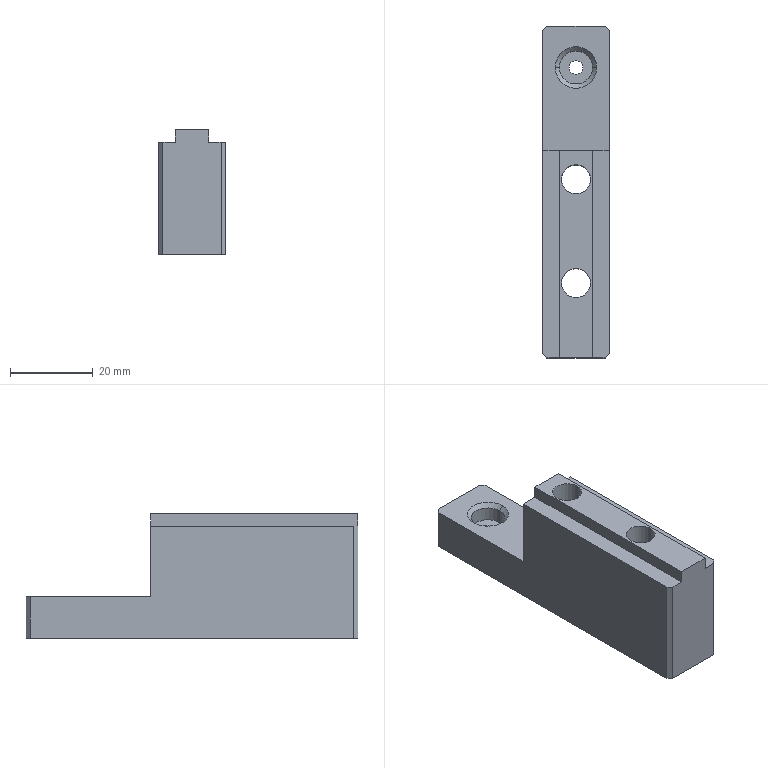Part | NX | features BREP 1 | 1 solid | 27 faces | box 16 x 80 x 30 mm | volume 24967 mm3 | plane 17 | cylinder 8 | cone 2 | commonest cylinder face diameters 7 x4 3.3 x2 8 x2
STEP:
#1=CARTESIAN_POINT('',(-3.5,3.,25.));
#2=VERTEX_POINT('',#1);
#3=CARTESIAN_POINT('',(3.5,3.,25.));
#4=VERTEX_POINT('',#3);
#5=CARTESIAN_POINT('',(0.,3.,25.));
#6=DIRECTION('',(0.,0.,1.));
#7=DIRECTION('',(-1.,0.,0.));
#8=AXIS2_PLACEMENT_3D('',#5,#6,#7);
#9=CIRCLE('',#8,3.5);
#10=EDGE_CURVE('',#2,#4,#9,.T.);
#11=ORIENTED_EDGE('',*,*,#10,.T.);
#12=CARTESIAN_POINT('',(3.5,3.,-5.));
#13=VERTEX_POINT('',#12);
#14=CARTESIAN_POINT('',(3.5,3.,25.));
#15=DIRECTION('',(0.,0.,-1.));
#16=VECTOR('',#15,1000.);
#17=LINE('',#14,#16);
#18=EDGE_CURVE('',#4,#13,#17,.T.);
#19=ORIENTED_EDGE('',*,*,#18,.T.);
#20=CARTESIAN_POINT('',(-3.5,3.,-5.));
#21=VERTEX_POINT('',#20);
#22=CARTESIAN_POINT('',(0.,3.,-5.));
#23=DIRECTION('',(0.,0.,1.));
#24=DIRECTION('',(1.,0.,0.));
#25=AXIS2_PLACEMENT_3D('',#22,#23,#24);
#26=CIRCLE('',#25,3.5);
#27=EDGE_CURVE('',#21,#13,#26,.T.);
#28=ORIENTED_EDGE('',*,*,#27,.F.);
#29=CARTESIAN_POINT('',(-3.5,3.,25.));
#30=DIRECTION('',(0.,0.,-1.));
#31=VECTOR('',#30,1000.);
#32=LINE('',#29,#31);
#33=EDGE_CURVE('',#2,#21,#32,.T.);
#34=ORIENTED_EDGE('',*,*,#33,.F.);
#35=EDGE_LOOP('',(#11,#19,#28,#34));
#36=FACE_BOUND('',#35,.T.);
#37=CARTESIAN_POINT('',(0.,3.,25.));
#38=DIRECTION('',(0.,0.,-1.));
#39=DIRECTION('',(-1.,0.,0.));
#40=AXIS2_PLACEMENT_3D('',#37,#38,#39);
#41=CYLINDRICAL_SURFACE('',#40,3.5);
#42=ADVANCED_FACE('',(#36),#41,.F.);
#43=CARTESIAN_POINT('',(-3.5,-22.,25.));
#44=VERTEX_POINT('',#43);
#45=CARTESIAN_POINT('',(3.5,-22.,25.));
#46=VERTEX_POINT('',#45);
#47=CARTESIAN_POINT('',(0.,-22.,25.));
#48=DIRECTION('',(0.,0.,1.));
#49=DIRECTION('',(-1.,0.,0.));
#50=AXIS2_PLACEMENT_3D('',#47,#48,#49);
#51=CIRCLE('',#50,3.5);
#52=EDGE_CURVE('',#44,#46,#51,.T.);
#53=ORIENTED_EDGE('',*,*,#52,.T.);
#54=CARTESIAN_POINT('',(3.5,-22.,-5.));
#55=VERTEX_POINT('',#54);
#56=CARTESIAN_POINT('',(3.5,-22.,25.));
#57=DIRECTION('',(0.,0.,-1.));
#58=VECTOR('',#57,1000.);
#59=LINE('',#56,#58);
#60=EDGE_CURVE('',#46,#55,#59,.T.);
#61=ORIENTED_EDGE('',*,*,#60,.T.);
#62=CARTESIAN_POINT('',(-3.5,-22.,-5.));
#63=VERTEX_POINT('',#62);
#64=CARTESIAN_POINT('',(0.,-22.,-5.));
#65=DIRECTION('',(0.,0.,1.));
#66=DIRECTION('',(1.,0.,0.));
#67=AXIS2_PLACEMENT_3D('',#64,#65,#66);
#68=CIRCLE('',#67,3.5);
#69=EDGE_CURVE('',#63,#55,#68,.T.);
#70=ORIENTED_EDGE('',*,*,#69,.F.);
#71=CARTESIAN_POINT('',(-3.5,-22.,25.));
#72=DIRECTION('',(0.,0.,-1.));
#73=VECTOR('',#72,1000.);
#74=LINE('',#71,#73);
#75=EDGE_CURVE('',#44,#63,#74,.T.);
#76=ORIENTED_EDGE('',*,*,#75,.F.);
#77=EDGE_LOOP('',(#53,#61,#70,#76));
#78=FACE_BOUND('',#77,.T.);
#79=CARTESIAN_POINT('',(0.,-22.,25.));
#80=DIRECTION('',(0.,0.,-1.));
#81=DIRECTION('',(-1.,0.,0.));
#82=AXIS2_PLACEMENT_3D('',#79,#80,#81);
#83=CYLINDRICAL_SURFACE('',#82,3.5);
#84=ADVANCED_FACE('',(#78),#83,.F.);
#85=CARTESIAN_POINT('',(-4.,30.,4.));
#86=VERTEX_POINT('',#85);
#87=CARTESIAN_POINT('',(4.,30.,4.));
#88=VERTEX_POINT('',#87);
#89=CARTESIAN_POINT('',(0.,30.,4.));
#90=DIRECTION('',(0.,0.,1.));
#91=DIRECTION('',(-1.,0.,0.));
#92=AXIS2_PLACEMENT_3D('',#89,#90,#91);
#93=CIRCLE('',#92,4.);
#94=EDGE_CURVE('',#86,#88,#93,.T.);
#95=ORIENTED_EDGE('',*,*,#94,.F.);
#96=CARTESIAN_POINT('',(-5.,30.,5.));
#97=VERTEX_POINT('',#96);
#98=CARTESIAN_POINT('',(-4.,30.,4.));
#99=DIRECTION('',(-0.7071,0.,0.7071));
#100=VECTOR('',#99,1000.);
#101=LINE('',#98,#100);
#102=EDGE_CURVE('',#97,#86,#101,.F.);
#103=ORIENTED_EDGE('',*,*,#102,.F.);
#104=CARTESIAN_POINT('',(5.,30.,5.));
#105=VERTEX_POINT('',#104);
#106=CARTESIAN_POINT('',(0.,30.,5.));
#107=DIRECTION('',(0.,0.,-1.));
#108=DIRECTION('',(-1.,0.,0.));
#109=AXIS2_PLACEMENT_3D('',#106,#107,#108);
#110=CIRCLE('',#109,5.);
#111=EDGE_CURVE('',#105,#97,#110,.T.);
#112=ORIENTED_EDGE('',*,*,#111,.F.);
#113=CARTESIAN_POINT('',(4.,30.,4.));
#114=DIRECTION('',(0.7071,0.,0.7071));
#115=VECTOR('',#114,1000.);
#116=LINE('',#113,#115);
#117=EDGE_CURVE('',#105,#88,#116,.F.);
#118=ORIENTED_EDGE('',*,*,#117,.T.);
#119=EDGE_LOOP('',(#95,#103,#112,#118));
#120=FACE_BOUND('',#119,.T.);
#121=CARTESIAN_POINT('',(0.,30.,4.));
#122=DIRECTION('',(0.,0.,1.));
#123=DIRECTION('',(1.,0.,0.));
#124=AXIS2_PLACEMENT_3D('',#121,#122,#123);
#125=CONICAL_SURFACE('',#124,4.,0.7854);
#126=ADVANCED_FACE('',(#120),#125,.F.);
#127=CARTESIAN_POINT('',(1.65,30.,-5.));
#128=VERTEX_POINT('',#127);
#129=CARTESIAN_POINT('',(-1.65,30.,-5.));
#130=VERTEX_POINT('',#129);
#131=CARTESIAN_POINT('',(0.,30.,-5.));
#132=DIRECTION('',(0.,0.,-1.));
#133=DIRECTION('',(-1.,0.,0.));
#134=AXIS2_PLACEMENT_3D('',#131,#132,#133);
#135=CIRCLE('',#134,1.65);
#136=EDGE_CURVE('',#128,#130,#135,.T.);
#137=ORIENTED_EDGE('',*,*,#136,.T.);
#138=CARTESIAN_POINT('',(-1.65,30.,0.5));
#139=VERTEX_POINT('',#138);
#140=CARTESIAN_POINT('',(-1.65,30.,0.5));
#141=DIRECTION('',(0.,0.,1.));
#142=VECTOR('',#141,1000.);
#143=LINE('',#140,#142);
#144=EDGE_CURVE('',#139,#130,#143,.F.);
#145=ORIENTED_EDGE('',*,*,#144,.F.);
#146=CARTESIAN_POINT('',(1.65,30.,0.5));
#147=VERTEX_POINT('',#146);
#148=CARTESIAN_POINT('',(0.,30.,0.5));
#149=DIRECTION('',(0.,0.,1.));
#150=DIRECTION('',(1.,0.,0.));
#151=AXIS2_PLACEMENT_3D('',#148,#149,#150);
#152=CIRCLE('',#151,1.65);
#153=EDGE_CURVE('',#139,#147,#152,.T.);
#154=ORIENTED_EDGE('',*,*,#153,.T.);
#155=CARTESIAN_POINT('',(1.65,30.,0.5));
#156=DIRECTION('',(0.,0.,1.));
#157=VECTOR('',#156,1000.);
#158=LINE('',#155,#157);
#159=EDGE_CURVE('',#147,#128,#158,.F.);
#160=ORIENTED_EDGE('',*,*,#159,.T.);
#161=EDGE_LOOP('',(#137,#145,#154,#160));
#162=FACE_BOUND('',#161,.T.);
#163=CARTESIAN_POINT('',(0.,30.,0.5));
#164=DIRECTION('',(0.,0.,1.));
#165=DIRECTION('',(1.,0.,0.));
#166=AXIS2_PLACEMENT_3D('',#163,#164,#165);
#167=CYLINDRICAL_SURFACE('',#166,1.65);
#168=ADVANCED_FACE('',(#162),#167,.F.);
#169=CARTESIAN_POINT('',(-4.,30.,0.5));
#170=VERTEX_POINT('',#169);
#171=CARTESIAN_POINT('',(4.,30.,0.5));
#172=VERTEX_POINT('',#171);
#173=CARTESIAN_POINT('',(0.,30.,0.5));
#174=DIRECTION('',(0.,0.,1.));
#175=DIRECTION('',(1.,0.,0.));
#176=AXIS2_PLACEMENT_3D('',#173,#174,#175);
#177=CIRCLE('',#176,4.);
#178=EDGE_CURVE('',#170,#172,#177,.T.);
#179=ORIENTED_EDGE('',*,*,#178,.F.);
#180=CARTESIAN_POINT('',(-4.,30.,0.5));
#181=DIRECTION('',(0.,0.,1.));
#182=VECTOR('',#181,1000.);
#183=LINE('',#180,#182);
#184=EDGE_CURVE('',#86,#170,#183,.F.);
#185=ORIENTED_EDGE('',*,*,#184,.F.);
#186=ORIENTED_EDGE('',*,*,#94,.T.);
#187=CARTESIAN_POINT('',(4.,30.,0.5));
#188=DIRECTION('',(0.,0.,1.));
#189=VECTOR('',#188,1000.);
#190=LINE('',#187,#189);
#191=EDGE_CURVE('',#88,#172,#190,.F.);
#192=ORIENTED_EDGE('',*,*,#191,.T.);
#193=EDGE_LOOP('',(#179,#185,#186,#192));
#194=FACE_BOUND('',#193,.T.);
#195=CARTESIAN_POINT('',(0.,30.,0.5));
#196=DIRECTION('',(0.,0.,1.));
#197=DIRECTION('',(1.,0.,0.));
#198=AXIS2_PLACEMENT_3D('',#195,#196,#197);
#199=CYLINDRICAL_SURFACE('',#198,4.);
#200=ADVANCED_FACE('',(#194),#199,.F.);
#201=CARTESIAN_POINT('',(-4.,10.,25.));
#202=VERTEX_POINT('',#201);
#203=CARTESIAN_POINT('',(-4.,-40.,25.));
#204=VERTEX_POINT('',#203);
#205=CARTESIAN_POINT('',(-4.,10.,25.));
#206=DIRECTION('',(0.,-1.,0.));
#207=VECTOR('',#206,1000.);
#208=LINE('',#205,#207);
#209=EDGE_CURVE('',#202,#204,#208,.T.);
#210=ORIENTED_EDGE('',*,*,#209,.T.);
#211=CARTESIAN_POINT('',(4.,-40.,25.));
#212=VERTEX_POINT('',#211);
#213=CARTESIAN_POINT('',(8.,-40.,25.));
#214=DIRECTION('',(1.,0.,0.));
#215=VECTOR('',#214,1000.);
#216=LINE('',#213,#215);
#217=EDGE_CURVE('',#204,#212,#216,.T.);
#218=ORIENTED_EDGE('',*,*,#217,.T.);
#219=CARTESIAN_POINT('',(4.,10.,25.));
#220=VERTEX_POINT('',#219);
#221=CARTESIAN_POINT('',(4.,10.,25.));
#222=DIRECTION('',(0.,1.,0.));
#223=VECTOR('',#222,1000.);
#224=LINE('',#221,#223);
#225=EDGE_CURVE('',#212,#220,#224,.T.);
#226=ORIENTED_EDGE('',*,*,#225,.T.);
#227=CARTESIAN_POINT('',(-8.,10.,25.));
#228=DIRECTION('',(-1.,0.,0.));
#229=VECTOR('',#228,1000.);
#230=LINE('',#227,#229);
#231=EDGE_CURVE('',#220,#202,#230,.T.);
#232=ORIENTED_EDGE('',*,*,#231,.T.);
#233=EDGE_LOOP('',(#210,#218,#226,#232));
#234=FACE_BOUND('',#233,.T.);
#235=ORIENTED_EDGE('',*,*,#52,.F.);
#236=CARTESIAN_POINT('',(0.,-22.,25.));
#237=DIRECTION('',(0.,0.,1.));
#238=DIRECTION('',(-1.,0.,0.));
#239=AXIS2_PLACEMENT_3D('',#236,#237,#238);
#240=CIRCLE('',#239,3.5);
#241=EDGE_CURVE('',#46,#44,#240,.T.);
#242=ORIENTED_EDGE('',*,*,#241,.F.);
#243=EDGE_LOOP('',(#235,#242));
#244=FACE_BOUND('',#243,.T.);
#245=ORIENTED_EDGE('',*,*,#10,.F.);
#246=CARTESIAN_POINT('',(0.,3.,25.));
#247=DIRECTION('',(0.,0.,1.));
#248=DIRECTION('',(-1.,0.,0.));
#249=AXIS2_PLACEMENT_3D('',#246,#247,#248);
#250=CIRCLE('',#249,3.5);
#251=EDGE_CURVE('',#4,#2,#250,.T.);
#252=ORIENTED_EDGE('',*,*,#251,.F.);
#253=EDGE_LOOP('',(#245,#252));
#254=FACE_BOUND('',#253,.T.);
#255=CARTESIAN_POINT('',(0.,0.,25.));
#256=DIRECTION('',(0.,0.,-1.));
#257=DIRECTION('',(0.,-1.,0.));
#258=AXIS2_PLACEMENT_3D('',#255,#256,#257);
#259=PLANE('',#258);
#260=ADVANCED_FACE('',(#234,#244,#254),#259,.F.);
#261=CARTESIAN_POINT('',(8.,-39.,22.));
#262=VERTEX_POINT('',#261);
#263=CARTESIAN_POINT('',(8.,10.,22.));
#264=VERTEX_POINT('',#263);
#265=CARTESIAN_POINT('',(8.,-40.,22.));
#266=DIRECTION('',(0.,1.,0.));
#267=VECTOR('',#266,1000.);
#268=LINE('',#265,#267);
#269=EDGE_CURVE('',#262,#264,#268,.T.);
#270=ORIENTED_EDGE('',*,*,#269,.F.);
#271=CARTESIAN_POINT('',(8.,-39.,-5.));
#272=VERTEX_POINT('',#271);
#273=CARTESIAN_POINT('',(8.,-39.,5.));
#274=DIRECTION('',(0.,0.,-1.));
#275=VECTOR('',#274,1000.);
#276=LINE('',#273,#275);
#277=EDGE_CURVE('',#262,#272,#276,.T.);
#278=ORIENTED_EDGE('',*,*,#277,.T.);
#279=CARTESIAN_POINT('',(8.,39.,-5.));
#280=VERTEX_POINT('',#279);
#281=CARTESIAN_POINT('',(8.,-40.,-5.));
#282=DIRECTION('',(0.,1.,0.));
#283=VECTOR('',#282,1000.);
#284=LINE('',#281,#283);
#285=EDGE_CURVE('',#272,#280,#284,.T.);
#286=ORIENTED_EDGE('',*,*,#285,.T.);
#287=CARTESIAN_POINT('',(8.,39.,5.));
#288=VERTEX_POINT('',#287);
#289=CARTESIAN_POINT('',(8.,39.,5.));
#290=DIRECTION('',(0.,0.,1.));
#291=VECTOR('',#290,1000.);
#292=LINE('',#289,#291);
#293=EDGE_CURVE('',#280,#288,#292,.T.);
#294=ORIENTED_EDGE('',*,*,#293,.T.);
#295=CARTESIAN_POINT('',(8.,10.,5.));
#296=VERTEX_POINT('',#295);
#297=CARTESIAN_POINT('',(8.,-40.,5.));
#298=DIRECTION('',(0.,1.,0.));
#299=VECTOR('',#298,1000.);
#300=LINE('',#297,#299);
#301=EDGE_CURVE('',#296,#288,#300,.T.);
#302=ORIENTED_EDGE('',*,*,#301,.F.);
#303=CARTESIAN_POINT('',(8.,10.,25.));
#304=DIRECTION('',(0.,0.,-1.));
#305=VECTOR('',#304,1000.);
#306=LINE('',#303,#305);
#307=EDGE_CURVE('',#264,#296,#306,.T.);
#308=ORIENTED_EDGE('',*,*,#307,.F.);
#309=EDGE_LOOP('',(#270,#278,#286,#294,#302,#308));
#310=FACE_BOUND('',#309,.T.);
#311=CARTESIAN_POINT('',(8.,-40.,5.));
#312=DIRECTION('',(-1.,0.,0.));
#313=DIRECTION('',(0.,0.,1.));
#314=AXIS2_PLACEMENT_3D('',#311,#312,#313);
#315=PLANE('',#314);
#316=ADVANCED_FACE('',(#310),#315,.F.);
#317=CARTESIAN_POINT('',(-8.,39.,-5.));
#318=VERTEX_POINT('',#317);
#319=CARTESIAN_POINT('',(-8.,-39.,-5.));
#320=VERTEX_POINT('',#319);
#321=CARTESIAN_POINT('',(-8.,-40.,-5.));
#322=DIRECTION('',(0.,-1.,0.));
#323=VECTOR('',#322,1000.);
#324=LINE('',#321,#323);
#325=EDGE_CURVE('',#318,#320,#324,.T.);
#326=ORIENTED_EDGE('',*,*,#325,.T.);
#327=CARTESIAN_POINT('',(-8.,-39.,22.));
#328=VERTEX_POINT('',#327);
#329=CARTESIAN_POINT('',(-8.,-39.,5.));
#330=DIRECTION('',(0.,0.,1.));
#331=VECTOR('',#330,1000.);
#332=LINE('',#329,#331);
#333=EDGE_CURVE('',#320,#328,#332,.T.);
#334=ORIENTED_EDGE('',*,*,#333,.T.);
#335=CARTESIAN_POINT('',(-8.,10.,22.));
#336=VERTEX_POINT('',#335);
#337=CARTESIAN_POINT('',(-8.,-40.,22.));
#338=DIRECTION('',(0.,-1.,0.));
#339=VECTOR('',#338,1000.);
#340=LINE('',#337,#339);
#341=EDGE_CURVE('',#336,#328,#340,.T.);
#342=ORIENTED_EDGE('',*,*,#341,.F.);
#343=CARTESIAN_POINT('',(-8.,10.,5.));
#344=VERTEX_POINT('',#343);
#345=CARTESIAN_POINT('',(-8.,10.,25.));
#346=DIRECTION('',(0.,0.,-1.));
#347=VECTOR('',#346,1000.);
#348=LINE('',#345,#347);
#349=EDGE_CURVE('',#336,#344,#348,.T.);
#350=ORIENTED_EDGE('',*,*,#349,.T.);
#351=CARTESIAN_POINT('',(-8.,39.,5.));
#352=VERTEX_POINT('',#351);
#353=CARTESIAN_POINT('',(-8.,-40.,5.));
#354=DIRECTION('',(0.,-1.,0.));
#355=VECTOR('',#354,1000.);
#356=LINE('',#353,#355);
#357=EDGE_CURVE('',#352,#344,#356,.T.);
#358=ORIENTED_EDGE('',*,*,#357,.F.);
#359=CARTESIAN_POINT('',(-8.,39.,5.));
#360=DIRECTION('',(0.,0.,-1.));
#361=VECTOR('',#360,1000.);
#362=LINE('',#359,#361);
#363=EDGE_CURVE('',#352,#318,#362,.T.);
#364=ORIENTED_EDGE('',*,*,#363,.T.);
#365=EDGE_LOOP('',(#326,#334,#342,#350,#358,#364));
#366=FACE_BOUND('',#365,.T.);
#367=CARTESIAN_POINT('',(-8.,-40.,5.));
#368=DIRECTION('',(1.,0.,0.));
#369=DIRECTION('',(0.,1.,0.));
#370=AXIS2_PLACEMENT_3D('',#367,#368,#369);
#371=PLANE('',#370);
#372=ADVANCED_FACE('',(#366),#371,.F.);
#373=CARTESIAN_POINT('',(-7.,-40.,22.));
#374=VERTEX_POINT('',#373);
#375=CARTESIAN_POINT('',(-4.,-40.,22.));
#376=VERTEX_POINT('',#375);
#377=CARTESIAN_POINT('',(-8.,-40.,22.));
#378=DIRECTION('',(1.,0.,0.));
#379=VECTOR('',#378,1000.);
#380=LINE('',#377,#379);
#381=EDGE_CURVE('',#374,#376,#380,.T.);
#382=ORIENTED_EDGE('',*,*,#381,.F.);
#383=CARTESIAN_POINT('',(-7.,-40.,-5.));
#384=VERTEX_POINT('',#383);
#385=CARTESIAN_POINT('',(-7.,-40.,5.));
#386=DIRECTION('',(0.,0.,-1.));
#387=VECTOR('',#386,1000.);
#388=LINE('',#385,#387);
#389=EDGE_CURVE('',#374,#384,#388,.T.);
#390=ORIENTED_EDGE('',*,*,#389,.T.);
#391=CARTESIAN_POINT('',(7.,-40.,-5.));
#392=VERTEX_POINT('',#391);
#393=CARTESIAN_POINT('',(-8.,-40.,-5.));
#394=DIRECTION('',(1.,0.,0.));
#395=VECTOR('',#394,1000.);
#396=LINE('',#393,#395);
#397=EDGE_CURVE('',#384,#392,#396,.T.);
#398=ORIENTED_EDGE('',*,*,#397,.T.);
#399=CARTESIAN_POINT('',(7.,-40.,22.));
#400=VERTEX_POINT('',#399);
#401=CARTESIAN_POINT('',(7.,-40.,5.));
#402=DIRECTION('',(0.,0.,1.));
#403=VECTOR('',#402,1000.);
#404=LINE('',#401,#403);
#405=EDGE_CURVE('',#392,#400,#404,.T.);
#406=ORIENTED_EDGE('',*,*,#405,.T.);
#407=CARTESIAN_POINT('',(4.,-40.,22.));
#408=VERTEX_POINT('',#407);
#409=CARTESIAN_POINT('',(-8.,-40.,22.));
#410=DIRECTION('',(1.,0.,0.));
#411=VECTOR('',#410,1000.);
#412=LINE('',#409,#411);
#413=EDGE_CURVE('',#408,#400,#412,.T.);
#414=ORIENTED_EDGE('',*,*,#413,.F.);
#415=CARTESIAN_POINT('',(4.,-40.,22.));
#416=DIRECTION('',(0.,0.,1.));
#417=VECTOR('',#416,1000.);
#418=LINE('',#415,#417);
#419=EDGE_CURVE('',#408,#212,#418,.T.);
#420=ORIENTED_EDGE('',*,*,#419,.T.);
#421=ORIENTED_EDGE('',*,*,#217,.F.);
#422=CARTESIAN_POINT('',(-4.,-40.,22.));
#423=DIRECTION('',(0.,0.,1.));
#424=VECTOR('',#423,1000.);
#425=LINE('',#422,#424);
#426=EDGE_CURVE('',#376,#204,#425,.T.);
#427=ORIENTED_EDGE('',*,*,#426,.F.);
#428=EDGE_LOOP('',(#382,#390,#398,#406,#414,#420,#421,#427));
#429=FACE_BOUND('',#428,.T.);
#430=CARTESIAN_POINT('',(-8.,-40.,5.));
#431=DIRECTION('',(0.,1.,0.));
#432=DIRECTION('',(1.,0.,0.));
#433=AXIS2_PLACEMENT_3D('',#430,#431,#432);
#434=PLANE('',#433);
#435=ADVANCED_FACE('',(#429),#434,.F.);
#436=CARTESIAN_POINT('',(-4.,10.,22.));
#437=VERTEX_POINT('',#436);
#438=CARTESIAN_POINT('',(-4.,10.,22.));
#439=DIRECTION('',(0.,0.,1.));
#440=VECTOR('',#439,1000.);
#441=LINE('',#438,#440);
#442=EDGE_CURVE('',#437,#202,#441,.T.);
#443=ORIENTED_EDGE('',*,*,#442,.T.);
#444=ORIENTED_EDGE('',*,*,#231,.F.);
#445=CARTESIAN_POINT('',(4.,10.,22.));
#446=VERTEX_POINT('',#445);
#447=CARTESIAN_POINT('',(4.,10.,22.));
#448=DIRECTION('',(0.,0.,1.));
#449=VECTOR('',#448,1000.);
#450=LINE('',#447,#449);
#451=EDGE_CURVE('',#446,#220,#450,.T.);
#452=ORIENTED_EDGE('',*,*,#451,.F.);
#453=CARTESIAN_POINT('',(-8.,10.,22.));
#454=DIRECTION('',(-1.,0.,0.));
#455=VECTOR('',#454,1000.);
#456=LINE('',#453,#455);
#457=EDGE_CURVE('',#264,#446,#456,.T.);
#458=ORIENTED_EDGE('',*,*,#457,.F.);
#459=ORIENTED_EDGE('',*,*,#307,.T.);
#460=CARTESIAN_POINT('',(-8.,10.,5.));
#461=DIRECTION('',(-1.,0.,0.));
#462=VECTOR('',#461,1000.);
#463=LINE('',#460,#462);
#464=EDGE_CURVE('',#296,#344,#463,.T.);
#465=ORIENTED_EDGE('',*,*,#464,.T.);
#466=ORIENTED_EDGE('',*,*,#349,.F.);
#467=CARTESIAN_POINT('',(-8.,10.,22.));
#468=DIRECTION('',(-1.,0.,0.));
#469=VECTOR('',#468,1000.);
#470=LINE('',#467,#469);
#471=EDGE_CURVE('',#437,#336,#470,.T.);
#472=ORIENTED_EDGE('',*,*,#471,.F.);
#473=EDGE_LOOP('',(#443,#444,#452,#458,#459,#465,#466,#472));
#474=FACE_BOUND('',#473,.T.);
#475=CARTESIAN_POINT('',(-8.,10.,25.));
#476=DIRECTION('',(0.,-1.,0.));
#477=DIRECTION('',(0.,0.,-1.));
#478=AXIS2_PLACEMENT_3D('',#475,#476,#477);
#479=PLANE('',#478);
#480=ADVANCED_FACE('',(#474),#479,.F.);
#481=ORIENTED_EDGE('',*,*,#397,.F.);
#482=CARTESIAN_POINT('',(-39.5,-7.5,-5.));
#483=DIRECTION('',(-0.7071,0.7071,0.));
#484=VECTOR('',#483,1000.);
#485=LINE('',#482,#484);
#486=EDGE_CURVE('',#384,#320,#485,.T.);
#487=ORIENTED_EDGE('',*,*,#486,.T.);
#488=ORIENTED_EDGE('',*,*,#325,.F.);
#489=CARTESIAN_POINT('',(-7.,40.,-5.));
#490=VERTEX_POINT('',#489);
#491=CARTESIAN_POINT('',(0.5,47.5,-5.));
#492=DIRECTION('',(0.7071,0.7071,0.));
#493=VECTOR('',#492,1000.);
#494=LINE('',#491,#493);
#495=EDGE_CURVE('',#318,#490,#494,.T.);
#496=ORIENTED_EDGE('',*,*,#495,.T.);
#497=CARTESIAN_POINT('',(7.,40.,-5.));
#498=VERTEX_POINT('',#497);
#499=CARTESIAN_POINT('',(-8.,40.,-5.));
#500=DIRECTION('',(-1.,0.,0.));
#501=VECTOR('',#500,1000.);
#502=LINE('',#499,#501);
#503=EDGE_CURVE('',#498,#490,#502,.T.);
#504=ORIENTED_EDGE('',*,*,#503,.F.);
#505=CARTESIAN_POINT('',(7.5,39.5,-5.));
#506=DIRECTION('',(0.7071,-0.7071,0.));
#507=VECTOR('',#506,1000.);
#508=LINE('',#505,#507);
#509=EDGE_CURVE('',#498,#280,#508,.T.);
#510=ORIENTED_EDGE('',*,*,#509,.T.);
#511=ORIENTED_EDGE('',*,*,#285,.F.);
#512=CARTESIAN_POINT('',(47.5,0.5,-5.));
#513=DIRECTION('',(-0.7071,-0.7071,0.));
#514=VECTOR('',#513,1000.);
#515=LINE('',#512,#514);
#516=EDGE_CURVE('',#272,#392,#515,.T.);
#517=ORIENTED_EDGE('',*,*,#516,.T.);
#518=EDGE_LOOP('',(#481,#487,#488,#496,#504,#510,#511,#517));
#519=FACE_BOUND('',#518,.T.);
#520=ORIENTED_EDGE('',*,*,#69,.T.);
#521=CARTESIAN_POINT('',(0.,-22.,-5.));
#522=DIRECTION('',(0.,0.,1.));
#523=DIRECTION('',(1.,0.,0.));
#524=AXIS2_PLACEMENT_3D('',#521,#522,#523);
#525=CIRCLE('',#524,3.5);
#526=EDGE_CURVE('',#55,#63,#525,.T.);
#527=ORIENTED_EDGE('',*,*,#526,.T.);
#528=EDGE_LOOP('',(#520,#527));
#529=FACE_BOUND('',#528,.T.);
#530=ORIENTED_EDGE('',*,*,#136,.F.);
#531=CARTESIAN_POINT('',(0.,30.,-5.));
#532=DIRECTION('',(0.,0.,-1.));
#533=DIRECTION('',(-1.,0.,0.));
#534=AXIS2_PLACEMENT_3D('',#531,#532,#533);
#535=CIRCLE('',#534,1.65);
#536=EDGE_CURVE('',#130,#128,#535,.T.);
#537=ORIENTED_EDGE('',*,*,#536,.F.);
#538=EDGE_LOOP('',(#530,#537));
#539=FACE_BOUND('',#538,.T.);
#540=ORIENTED_EDGE('',*,*,#27,.T.);
#541=CARTESIAN_POINT('',(0.,3.,-5.));
#542=DIRECTION('',(0.,0.,1.));
#543=DIRECTION('',(1.,0.,0.));
#544=AXIS2_PLACEMENT_3D('',#541,#542,#543);
#545=CIRCLE('',#544,3.5);
#546=EDGE_CURVE('',#13,#21,#545,.T.);
#547=ORIENTED_EDGE('',*,*,#546,.T.);
#548=EDGE_LOOP('',(#540,#547));
#549=FACE_BOUND('',#548,.T.);
#550=CARTESIAN_POINT('',(8.,40.,-5.));
#551=DIRECTION('',(0.,0.,-1.));
#552=DIRECTION('',(0.,-1.,0.));
#553=AXIS2_PLACEMENT_3D('',#550,#551,#552);
#554=PLANE('',#553);
#555=ADVANCED_FACE('',(#519,#529,#539,#549),#554,.T.);
#556=ORIENTED_EDGE('',*,*,#301,.T.);
#557=CARTESIAN_POINT('',(7.,40.,5.));
#558=VERTEX_POINT('',#557);
#559=CARTESIAN_POINT('',(7.,40.,5.));
#560=DIRECTION('',(-0.7071,0.7071,0.));
#561=VECTOR('',#560,1000.);
#562=LINE('',#559,#561);
#563=EDGE_CURVE('',#288,#558,#562,.T.);
#564=ORIENTED_EDGE('',*,*,#563,.T.);
#565=CARTESIAN_POINT('',(-7.,40.,5.));
#566=VERTEX_POINT('',#565);
#567=CARTESIAN_POINT('',(-8.,40.,5.));
#568=DIRECTION('',(-1.,0.,0.));
#569=VECTOR('',#568,1000.);
#570=LINE('',#567,#569);
#571=EDGE_CURVE('',#558,#566,#570,.T.);
#572=ORIENTED_EDGE('',*,*,#571,.T.);
#573=CARTESIAN_POINT('',(-8.,39.,5.));
#574=DIRECTION('',(-0.7071,-0.7071,0.));
#575=VECTOR('',#574,1000.);
#576=LINE('',#573,#575);
#577=EDGE_CURVE('',#566,#352,#576,.T.);
#578=ORIENTED_EDGE('',*,*,#577,.T.);
#579=ORIENTED_EDGE('',*,*,#357,.T.);
#580=ORIENTED_EDGE('',*,*,#464,.F.);
#581=EDGE_LOOP('',(#556,#564,#572,#578,#579,#580));
#582=FACE_BOUND('',#581,.T.);
#583=ORIENTED_EDGE('',*,*,#111,.T.);
#584=CARTESIAN_POINT('',(0.,30.,5.));
#585=DIRECTION('',(0.,0.,-1.));
#586=DIRECTION('',(-1.,0.,0.));
#587=AXIS2_PLACEMENT_3D('',#584,#585,#586);
#588=CIRCLE('',#587,5.);
#589=EDGE_CURVE('',#97,#105,#588,.T.);
#590=ORIENTED_EDGE('',*,*,#589,.T.);
#591=EDGE_LOOP('',(#583,#590));
#592=FACE_BOUND('',#591,.T.);
#593=CARTESIAN_POINT('',(8.,40.,5.));
#594=DIRECTION('',(0.,0.,-1.));
#595=DIRECTION('',(0.,-1.,0.));
#596=AXIS2_PLACEMENT_3D('',#593,#594,#595);
#597=PLANE('',#596);
#598=ADVANCED_FACE('',(#582,#592),#597,.F.);
#599=ORIENTED_EDGE('',*,*,#571,.F.);
#600=CARTESIAN_POINT('',(7.,40.,5.));
#601=DIRECTION('',(0.,0.,-1.));
#602=VECTOR('',#601,1000.);
#603=LINE('',#600,#602);
#604=EDGE_CURVE('',#558,#498,#603,.T.);
#605=ORIENTED_EDGE('',*,*,#604,.T.);
#606=ORIENTED_EDGE('',*,*,#503,.T.);
#607=CARTESIAN_POINT('',(-7.,40.,5.));
#608=DIRECTION('',(0.,0.,1.));
#609=VECTOR('',#608,1000.);
#610=LINE('',#607,#609);
#611=EDGE_CURVE('',#490,#566,#610,.T.);
#612=ORIENTED_EDGE('',*,*,#611,.T.);
#613=EDGE_LOOP('',(#599,#605,#606,#612));
#614=FACE_BOUND('',#613,.T.);
#615=CARTESIAN_POINT('',(-8.,40.,5.));
#616=DIRECTION('',(0.,-1.,0.));
#617=DIRECTION('',(0.,0.,-1.));
#618=AXIS2_PLACEMENT_3D('',#615,#616,#617);
#619=PLANE('',#618);
#620=ADVANCED_FACE('',(#614),#619,.F.);
#621=ORIENTED_EDGE('',*,*,#184,.T.);
#622=CARTESIAN_POINT('',(0.,30.,0.5));
#623=DIRECTION('',(0.,0.,1.));
#624=DIRECTION('',(1.,0.,0.));
#625=AXIS2_PLACEMENT_3D('',#622,#623,#624);
#626=CIRCLE('',#625,4.);
#627=EDGE_CURVE('',#172,#170,#626,.T.);
#628=ORIENTED_EDGE('',*,*,#627,.F.);
#629=ORIENTED_EDGE('',*,*,#191,.F.);
#630=CARTESIAN_POINT('',(0.,30.,4.));
#631=DIRECTION('',(0.,0.,1.));
#632=DIRECTION('',(-1.,0.,0.));
#633=AXIS2_PLACEMENT_3D('',#630,#631,#632);
#634=CIRCLE('',#633,4.);
#635=EDGE_CURVE('',#88,#86,#634,.T.);
#636=ORIENTED_EDGE('',*,*,#635,.T.);
#637=EDGE_LOOP('',(#621,#628,#629,#636));
#638=FACE_BOUND('',#637,.T.);
#639=CARTESIAN_POINT('',(0.,30.,0.5));
#640=DIRECTION('',(0.,0.,1.));
#641=DIRECTION('',(1.,0.,0.));
#642=AXIS2_PLACEMENT_3D('',#639,#640,#641);
#643=CYLINDRICAL_SURFACE('',#642,4.);
#644=ADVANCED_FACE('',(#638),#643,.F.);
#645=ORIENTED_EDGE('',*,*,#627,.T.);
#646=ORIENTED_EDGE('',*,*,#178,.T.);
#647=EDGE_LOOP('',(#645,#646));
#648=FACE_BOUND('',#647,.T.);
#649=CARTESIAN_POINT('',(0.,30.,0.5));
#650=DIRECTION('',(0.,0.,1.));
#651=DIRECTION('',(1.,0.,0.));
#652=AXIS2_PLACEMENT_3D('',#649,#650,#651);
#653=CIRCLE('',#652,1.65);
#654=EDGE_CURVE('',#147,#139,#653,.T.);
#655=ORIENTED_EDGE('',*,*,#654,.F.);
#656=ORIENTED_EDGE('',*,*,#153,.F.);
#657=EDGE_LOOP('',(#655,#656));
#658=FACE_BOUND('',#657,.T.);
#659=CARTESIAN_POINT('',(0.,30.,0.5));
#660=DIRECTION('',(0.,0.,1.));
#661=DIRECTION('',(1.,0.,0.));
#662=AXIS2_PLACEMENT_3D('',#659,#660,#661);
#663=PLANE('',#662);
#664=ADVANCED_FACE('',(#648,#658),#663,.T.);
#665=ORIENTED_EDGE('',*,*,#144,.T.);
#666=ORIENTED_EDGE('',*,*,#536,.T.);
#667=ORIENTED_EDGE('',*,*,#159,.F.);
#668=ORIENTED_EDGE('',*,*,#654,.T.);
#669=EDGE_LOOP('',(#665,#666,#667,#668));
#670=FACE_BOUND('',#669,.T.);
#671=CARTESIAN_POINT('',(0.,30.,0.5));
#672=DIRECTION('',(0.,0.,1.));
#673=DIRECTION('',(1.,0.,0.));
#674=AXIS2_PLACEMENT_3D('',#671,#672,#673);
#675=CYLINDRICAL_SURFACE('',#674,1.65);
#676=ADVANCED_FACE('',(#670),#675,.F.);
#677=ORIENTED_EDGE('',*,*,#102,.T.);
#678=ORIENTED_EDGE('',*,*,#635,.F.);
#679=ORIENTED_EDGE('',*,*,#117,.F.);
#680=ORIENTED_EDGE('',*,*,#589,.F.);
#681=EDGE_LOOP('',(#677,#678,#679,#680));
#682=FACE_BOUND('',#681,.T.);
#683=CARTESIAN_POINT('',(0.,30.,4.));
#684=DIRECTION('',(0.,0.,1.));
#685=DIRECTION('',(1.,0.,0.));
#686=AXIS2_PLACEMENT_3D('',#683,#684,#685);
#687=CONICAL_SURFACE('',#686,4.,0.7854);
#688=ADVANCED_FACE('',(#682),#687,.F.);
#689=ORIENTED_EDGE('',*,*,#60,.F.);
#690=ORIENTED_EDGE('',*,*,#241,.T.);
#691=ORIENTED_EDGE('',*,*,#75,.T.);
#692=ORIENTED_EDGE('',*,*,#526,.F.);
#693=EDGE_LOOP('',(#689,#690,#691,#692));
#694=FACE_BOUND('',#693,.T.);
#695=CARTESIAN_POINT('',(0.,-22.,25.));
#696=DIRECTION('',(0.,0.,-1.));
#697=DIRECTION('',(-1.,0.,0.));
#698=AXIS2_PLACEMENT_3D('',#695,#696,#697);
#699=CYLINDRICAL_SURFACE('',#698,3.5);
#700=ADVANCED_FACE('',(#694),#699,.F.);
#701=ORIENTED_EDGE('',*,*,#18,.F.);
#702=ORIENTED_EDGE('',*,*,#251,.T.);
#703=ORIENTED_EDGE('',*,*,#33,.T.);
#704=ORIENTED_EDGE('',*,*,#546,.F.);
#705=EDGE_LOOP('',(#701,#702,#703,#704));
#706=FACE_BOUND('',#705,.T.);
#707=CARTESIAN_POINT('',(0.,3.,25.));
#708=DIRECTION('',(0.,0.,-1.));
#709=DIRECTION('',(-1.,0.,0.));
#710=AXIS2_PLACEMENT_3D('',#707,#708,#709);
#711=CYLINDRICAL_SURFACE('',#710,3.5);
#712=ADVANCED_FACE('',(#706),#711,.F.);
#713=ORIENTED_EDGE('',*,*,#225,.F.);
#714=ORIENTED_EDGE('',*,*,#419,.F.);
#715=CARTESIAN_POINT('',(4.,10.,22.));
#716=DIRECTION('',(0.,1.,0.));
#717=VECTOR('',#716,1000.);
#718=LINE('',#715,#717);
#719=EDGE_CURVE('',#408,#446,#718,.T.);
#720=ORIENTED_EDGE('',*,*,#719,.T.);
#721=ORIENTED_EDGE('',*,*,#451,.T.);
#722=EDGE_LOOP('',(#713,#714,#720,#721));
#723=FACE_BOUND('',#722,.T.);
#724=CARTESIAN_POINT('',(4.,10.,22.));
#725=DIRECTION('',(1.,0.,0.));
#726=DIRECTION('',(0.,-1.,0.));
#727=AXIS2_PLACEMENT_3D('',#724,#725,#726);
#728=PLANE('',#727);
#729=ADVANCED_FACE('',(#723),#728,.T.);
#730=ORIENTED_EDGE('',*,*,#413,.T.);
#731=CARTESIAN_POINT('',(23.5,-23.5,22.));
#732=DIRECTION('',(0.7071,0.7071,0.));
#733=VECTOR('',#732,1000.);
#734=LINE('',#731,#733);
#735=EDGE_CURVE('',#400,#262,#734,.T.);
#736=ORIENTED_EDGE('',*,*,#735,.T.);
#737=ORIENTED_EDGE('',*,*,#269,.T.);
#738=ORIENTED_EDGE('',*,*,#457,.T.);
#739=ORIENTED_EDGE('',*,*,#719,.F.);
#740=EDGE_LOOP('',(#730,#736,#737,#738,#739));
#741=FACE_BOUND('',#740,.T.);
#742=CARTESIAN_POINT('',(0.,0.0000125,22.));
#743=DIRECTION('',(0.,0.,1.));
#744=DIRECTION('',(1.,0.,0.));
#745=AXIS2_PLACEMENT_3D('',#742,#743,#744);
#746=PLANE('',#745);
#747=ADVANCED_FACE('',(#741),#746,.T.);
#748=ORIENTED_EDGE('',*,*,#341,.T.);
#749=CARTESIAN_POINT('',(-23.5,-23.5,22.));
#750=DIRECTION('',(0.7071,-0.7071,0.));
#751=VECTOR('',#750,1000.);
#752=LINE('',#749,#751);
#753=EDGE_CURVE('',#328,#374,#752,.T.);
#754=ORIENTED_EDGE('',*,*,#753,.T.);
#755=ORIENTED_EDGE('',*,*,#381,.T.);
#756=CARTESIAN_POINT('',(-4.,10.,22.));
#757=DIRECTION('',(0.,-1.,0.));
#758=VECTOR('',#757,1000.);
#759=LINE('',#756,#758);
#760=EDGE_CURVE('',#437,#376,#759,.T.);
#761=ORIENTED_EDGE('',*,*,#760,.F.);
#762=ORIENTED_EDGE('',*,*,#471,.T.);
#763=EDGE_LOOP('',(#748,#754,#755,#761,#762));
#764=FACE_BOUND('',#763,.T.);
#765=CARTESIAN_POINT('',(0.,0.0000125,22.));
#766=DIRECTION('',(0.,0.,1.));
#767=DIRECTION('',(1.,0.,0.));
#768=AXIS2_PLACEMENT_3D('',#765,#766,#767);
#769=PLANE('',#768);
#770=ADVANCED_FACE('',(#764),#769,.T.);
#771=ORIENTED_EDGE('',*,*,#209,.F.);
#772=ORIENTED_EDGE('',*,*,#442,.F.);
#773=ORIENTED_EDGE('',*,*,#760,.T.);
#774=ORIENTED_EDGE('',*,*,#426,.T.);
#775=EDGE_LOOP('',(#771,#772,#773,#774));
#776=FACE_BOUND('',#775,.T.);
#777=CARTESIAN_POINT('',(-4.,10.,22.));
#778=DIRECTION('',(-1.,0.,0.));
#779=DIRECTION('',(0.,1.,0.));
#780=AXIS2_PLACEMENT_3D('',#777,#778,#779);
#781=PLANE('',#780);
#782=ADVANCED_FACE('',(#776),#781,.T.);
#783=ORIENTED_EDGE('',*,*,#753,.F.);
#784=ORIENTED_EDGE('',*,*,#333,.F.);
#785=ORIENTED_EDGE('',*,*,#486,.F.);
#786=ORIENTED_EDGE('',*,*,#389,.F.);
#787=EDGE_LOOP('',(#783,#784,#785,#786));
#788=FACE_BOUND('',#787,.T.);
#789=CARTESIAN_POINT('',(-7.,-40.,5.));
#790=DIRECTION('',(0.7071,0.7071,0.));
#791=DIRECTION('',(0.,0.,-1.));
#792=AXIS2_PLACEMENT_3D('',#789,#790,#791);
#793=PLANE('',#792);
#794=ADVANCED_FACE('',(#788),#793,.F.);
#795=ORIENTED_EDGE('',*,*,#735,.F.);
#796=ORIENTED_EDGE('',*,*,#405,.F.);
#797=ORIENTED_EDGE('',*,*,#516,.F.);
#798=ORIENTED_EDGE('',*,*,#277,.F.);
#799=EDGE_LOOP('',(#795,#796,#797,#798));
#800=FACE_BOUND('',#799,.T.);
#801=CARTESIAN_POINT('',(8.,-39.,5.));
#802=DIRECTION('',(-0.7071,0.7071,0.));
#803=DIRECTION('',(0.,0.,1.));
#804=AXIS2_PLACEMENT_3D('',#801,#802,#803);
#805=PLANE('',#804);
#806=ADVANCED_FACE('',(#800),#805,.F.);
#807=ORIENTED_EDGE('',*,*,#563,.F.);
#808=ORIENTED_EDGE('',*,*,#293,.F.);
#809=ORIENTED_EDGE('',*,*,#509,.F.);
#810=ORIENTED_EDGE('',*,*,#604,.F.);
#811=EDGE_LOOP('',(#807,#808,#809,#810));
#812=FACE_BOUND('',#811,.T.);
#813=CARTESIAN_POINT('',(7.,40.,5.));
#814=DIRECTION('',(-0.7071,-0.7071,0.));
#815=DIRECTION('',(-0.7071,0.7071,0.));
#816=AXIS2_PLACEMENT_3D('',#813,#814,#815);
#817=PLANE('',#816);
#818=ADVANCED_FACE('',(#812),#817,.F.);
#819=ORIENTED_EDGE('',*,*,#577,.F.);
#820=ORIENTED_EDGE('',*,*,#611,.F.);
#821=ORIENTED_EDGE('',*,*,#495,.F.);
#822=ORIENTED_EDGE('',*,*,#363,.F.);
#823=EDGE_LOOP('',(#819,#820,#821,#822));
#824=FACE_BOUND('',#823,.T.);
#825=CARTESIAN_POINT('',(-8.,39.,5.));
#826=DIRECTION('',(0.7071,-0.7071,0.));
#827=DIRECTION('',(0.,0.,-1.));
#828=AXIS2_PLACEMENT_3D('',#825,#826,#827);
#829=PLANE('',#828);
#830=ADVANCED_FACE('',(#824),#829,.F.);
#831=CLOSED_SHELL('',(#42,#84,#126,#168,#200,#260,#316,#372,#435,#480,#555,#598,#620,#644,#664,#676,#688,#700,#712,#729,#747,#770,#782,#794,#806,#818,#830));
#832=MANIFOLD_SOLID_BREP('',#831);
#833=(LENGTH_UNIT()NAMED_UNIT(*)SI_UNIT(.MILLI.,.METRE.));
#834=UNCERTAINTY_MEASURE_WITH_UNIT(LENGTH_MEASURE(0.00001),#833,'','');
#835=(NAMED_UNIT(*)PLANE_ANGLE_UNIT()SI_UNIT($,.RADIAN.));
#836=(NAMED_UNIT(*)SI_UNIT($,.STERADIAN.)SOLID_ANGLE_UNIT());
#837=(GEOMETRIC_REPRESENTATION_CONTEXT(3)GLOBAL_UNCERTAINTY_ASSIGNED_CONTEXT((#834))GLOBAL_UNIT_ASSIGNED_CONTEXT((#833,#835,#836))REPRESENTATION_CONTEXT('',''));
#838=ADVANCED_BREP_SHAPE_REPRESENTATION('',(#832),#837);